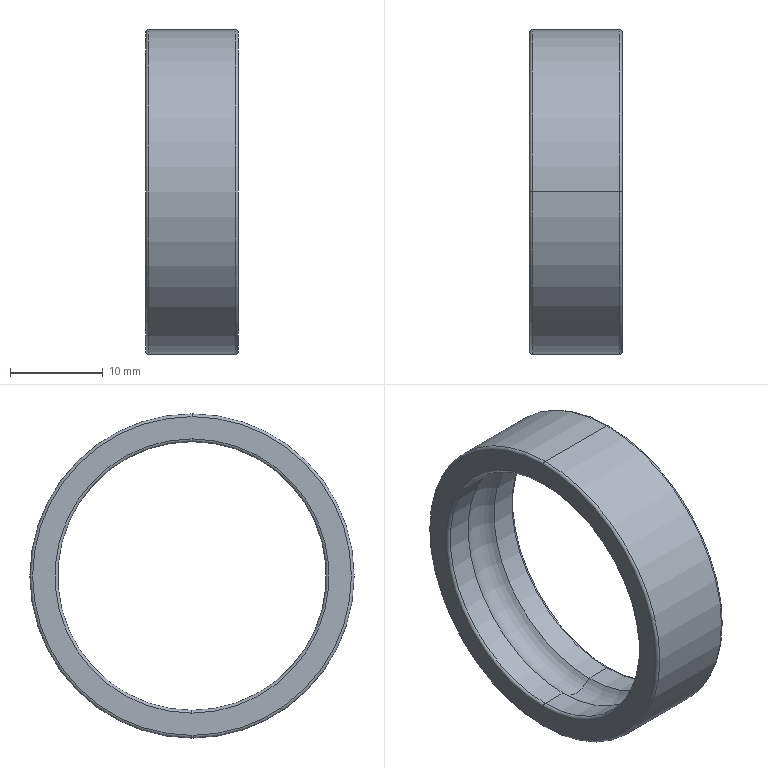Part | SolidWorks | features BaseBody 1 | 1 solid | 18 faces | box 10 x 35 x 35 mm | volume 2757 mm3 | torus 10 | cylinder 6 | plane 2 | commonest cylinder face diameters 29 x4 35 x2
STEP:
#1=CARTESIAN_POINT('',(1.969,0.,14.5));
#2=VERTEX_POINT('',#1);
#3=CARTESIAN_POINT('',(1.969,0.,-14.5));
#4=VERTEX_POINT('',#3);
#5=CARTESIAN_POINT('',(1.969,0.,0.));
#6=DIRECTION('',(1.,0.,0.));
#7=DIRECTION('',(0.,0.,1.));
#8=AXIS2_PLACEMENT_3D('',#5,#6,#7);
#9=CIRCLE('',#8,14.5);
#10=EDGE_CURVE('',#2,#4,#9,.T.);
#11=ORIENTED_EDGE('',*,*,#10,.T.);
#12=CARTESIAN_POINT('',(-1.969,0.,-14.5));
#13=VERTEX_POINT('',#12);
#14=CARTESIAN_POINT('',(0.,0.,-13.));
#15=DIRECTION('',(0.,1.,0.));
#16=DIRECTION('',(0.,0.,1.));
#17=AXIS2_PLACEMENT_3D('',#14,#15,#16);
#18=CIRCLE('',#17,2.475);
#19=EDGE_CURVE('',#4,#13,#18,.T.);
#20=ORIENTED_EDGE('',*,*,#19,.T.);
#21=CARTESIAN_POINT('',(-1.969,0.,14.5));
#22=VERTEX_POINT('',#21);
#23=CARTESIAN_POINT('',(-1.969,0.,0.));
#24=DIRECTION('',(-1.,0.,0.));
#25=DIRECTION('',(0.,0.,-1.));
#26=AXIS2_PLACEMENT_3D('',#23,#24,#25);
#27=CIRCLE('',#26,14.5);
#28=EDGE_CURVE('',#13,#22,#27,.T.);
#29=ORIENTED_EDGE('',*,*,#28,.T.);
#30=CARTESIAN_POINT('',(0.,0.,13.));
#31=DIRECTION('',(0.,-1.,0.));
#32=DIRECTION('',(0.,0.,-1.));
#33=AXIS2_PLACEMENT_3D('',#30,#31,#32);
#34=CIRCLE('',#33,2.475);
#35=EDGE_CURVE('',#2,#22,#34,.T.);
#36=ORIENTED_EDGE('',*,*,#35,.F.);
#37=EDGE_LOOP('',(#11,#20,#29,#36));
#38=FACE_OUTER_BOUND('',#37,.T.);
#39=CARTESIAN_POINT('',(0.,0.,0.));
#40=DIRECTION('',(-1.,0.,0.));
#41=DIRECTION('',(0.,0.,1.));
#42=AXIS2_PLACEMENT_3D('',#39,#40,#41);
#43=TOROIDAL_SURFACE('',#42,13.,2.475);
#44=ADVANCED_FACE('',(#38),#43,.F.);
#45=CARTESIAN_POINT('',(4.7,0.,17.5));
#46=VERTEX_POINT('',#45);
#47=CARTESIAN_POINT('',(4.7,0.,-17.5));
#48=VERTEX_POINT('',#47);
#49=CARTESIAN_POINT('',(4.7,0.,0.));
#50=DIRECTION('',(-1.,0.,0.));
#51=DIRECTION('',(0.,0.,1.));
#52=AXIS2_PLACEMENT_3D('',#49,#50,#51);
#53=CIRCLE('',#52,17.5);
#54=EDGE_CURVE('',#46,#48,#53,.T.);
#55=ORIENTED_EDGE('',*,*,#54,.T.);
#56=CARTESIAN_POINT('',(-4.7,0.,-17.5));
#57=VERTEX_POINT('',#56);
#58=CARTESIAN_POINT('',(-3.5,0.,-17.5));
#59=DIRECTION('',(-1.,0.,0.));
#60=VECTOR('',#59,1000.);
#61=LINE('',#58,#60);
#62=EDGE_CURVE('',#48,#57,#61,.T.);
#63=ORIENTED_EDGE('',*,*,#62,.T.);
#64=CARTESIAN_POINT('',(-4.7,0.,17.5));
#65=VERTEX_POINT('',#64);
#66=CARTESIAN_POINT('',(-4.7,0.,0.));
#67=DIRECTION('',(-1.,0.,0.));
#68=DIRECTION('',(0.,0.,1.));
#69=AXIS2_PLACEMENT_3D('',#66,#67,#68);
#70=CIRCLE('',#69,17.5);
#71=EDGE_CURVE('',#65,#57,#70,.T.);
#72=ORIENTED_EDGE('',*,*,#71,.F.);
#73=CARTESIAN_POINT('',(-3.5,0.,17.5));
#74=DIRECTION('',(-1.,0.,0.));
#75=VECTOR('',#74,1000.);
#76=LINE('',#73,#75);
#77=EDGE_CURVE('',#46,#65,#76,.T.);
#78=ORIENTED_EDGE('',*,*,#77,.F.);
#79=EDGE_LOOP('',(#55,#63,#72,#78));
#80=FACE_OUTER_BOUND('',#79,.T.);
#81=CARTESIAN_POINT('',(-3.5,0.,0.));
#82=DIRECTION('',(-1.,0.,0.));
#83=DIRECTION('',(0.,0.,1.));
#84=AXIS2_PLACEMENT_3D('',#81,#82,#83);
#85=CYLINDRICAL_SURFACE('',#84,17.5);
#86=ADVANCED_FACE('',(#80),#85,.T.);
#87=CARTESIAN_POINT('',(5.,0.,17.2));
#88=VERTEX_POINT('',#87);
#89=CARTESIAN_POINT('',(5.,0.,-17.2));
#90=VERTEX_POINT('',#89);
#91=CARTESIAN_POINT('',(5.,0.,0.));
#92=DIRECTION('',(-1.,0.,0.));
#93=DIRECTION('',(0.,0.,1.));
#94=AXIS2_PLACEMENT_3D('',#91,#92,#93);
#95=CIRCLE('',#94,17.2);
#96=EDGE_CURVE('',#88,#90,#95,.T.);
#97=ORIENTED_EDGE('',*,*,#96,.T.);
#98=CARTESIAN_POINT('',(4.7,0.,-17.2));
#99=DIRECTION('',(0.,1.,0.));
#100=DIRECTION('',(0.,0.,1.));
#101=AXIS2_PLACEMENT_3D('',#98,#99,#100);
#102=CIRCLE('',#101,0.3);
#103=EDGE_CURVE('',#90,#48,#102,.T.);
#104=ORIENTED_EDGE('',*,*,#103,.T.);
#105=ORIENTED_EDGE('',*,*,#54,.F.);
#106=CARTESIAN_POINT('',(4.7,0.,17.2));
#107=DIRECTION('',(0.,-1.,0.));
#108=DIRECTION('',(0.,0.,-1.));
#109=AXIS2_PLACEMENT_3D('',#106,#107,#108);
#110=CIRCLE('',#109,0.3);
#111=EDGE_CURVE('',#88,#46,#110,.T.);
#112=ORIENTED_EDGE('',*,*,#111,.F.);
#113=EDGE_LOOP('',(#97,#104,#105,#112));
#114=FACE_OUTER_BOUND('',#113,.T.);
#115=CARTESIAN_POINT('',(4.7,0.,0.));
#116=DIRECTION('',(-1.,0.,0.));
#117=DIRECTION('',(0.,0.,1.));
#118=AXIS2_PLACEMENT_3D('',#115,#116,#117);
#119=TOROIDAL_SURFACE('',#118,17.2,0.3);
#120=ADVANCED_FACE('',(#114),#119,.T.);
#121=CARTESIAN_POINT('',(4.7,0.,14.5));
#122=VERTEX_POINT('',#121);
#123=CARTESIAN_POINT('',(4.7,0.,-14.5));
#124=VERTEX_POINT('',#123);
#125=CARTESIAN_POINT('',(4.7,0.,0.));
#126=DIRECTION('',(-1.,0.,0.));
#127=DIRECTION('',(0.,0.,1.));
#128=AXIS2_PLACEMENT_3D('',#125,#126,#127);
#129=CIRCLE('',#128,14.5);
#130=EDGE_CURVE('',#122,#124,#129,.T.);
#131=ORIENTED_EDGE('',*,*,#130,.T.);
#132=CARTESIAN_POINT('',(5.,0.,-14.8));
#133=VERTEX_POINT('',#132);
#134=CARTESIAN_POINT('',(4.7,0.,-14.8));
#135=DIRECTION('',(0.,1.,0.));
#136=DIRECTION('',(0.,0.,1.));
#137=AXIS2_PLACEMENT_3D('',#134,#135,#136);
#138=CIRCLE('',#137,0.3);
#139=EDGE_CURVE('',#124,#133,#138,.T.);
#140=ORIENTED_EDGE('',*,*,#139,.T.);
#141=CARTESIAN_POINT('',(5.,0.,14.8));
#142=VERTEX_POINT('',#141);
#143=CARTESIAN_POINT('',(5.,0.,0.));
#144=DIRECTION('',(-1.,0.,0.));
#145=DIRECTION('',(0.,0.,1.));
#146=AXIS2_PLACEMENT_3D('',#143,#144,#145);
#147=CIRCLE('',#146,14.8);
#148=EDGE_CURVE('',#142,#133,#147,.T.);
#149=ORIENTED_EDGE('',*,*,#148,.F.);
#150=CARTESIAN_POINT('',(4.7,0.,14.8));
#151=DIRECTION('',(0.,-1.,0.));
#152=DIRECTION('',(0.,0.,-1.));
#153=AXIS2_PLACEMENT_3D('',#150,#151,#152);
#154=CIRCLE('',#153,0.3);
#155=EDGE_CURVE('',#122,#142,#154,.T.);
#156=ORIENTED_EDGE('',*,*,#155,.F.);
#157=EDGE_LOOP('',(#131,#140,#149,#156));
#158=FACE_OUTER_BOUND('',#157,.T.);
#159=CARTESIAN_POINT('',(4.7,0.,0.));
#160=DIRECTION('',(-1.,0.,0.));
#161=DIRECTION('',(0.,0.,1.));
#162=AXIS2_PLACEMENT_3D('',#159,#160,#161);
#163=TOROIDAL_SURFACE('',#162,14.8,0.3);
#164=ADVANCED_FACE('',(#158),#163,.T.);
#165=CARTESIAN_POINT('',(-5.,0.,14.8));
#166=VERTEX_POINT('',#165);
#167=CARTESIAN_POINT('',(-5.,0.,-14.8));
#168=VERTEX_POINT('',#167);
#169=CARTESIAN_POINT('',(-5.,0.,0.));
#170=DIRECTION('',(-1.,0.,0.));
#171=DIRECTION('',(0.,0.,1.));
#172=AXIS2_PLACEMENT_3D('',#169,#170,#171);
#173=CIRCLE('',#172,14.8);
#174=EDGE_CURVE('',#166,#168,#173,.T.);
#175=ORIENTED_EDGE('',*,*,#174,.T.);
#176=CARTESIAN_POINT('',(-4.7,0.,-14.5));
#177=VERTEX_POINT('',#176);
#178=CARTESIAN_POINT('',(-4.7,0.,-14.8));
#179=DIRECTION('',(0.,1.,0.));
#180=DIRECTION('',(0.,0.,1.));
#181=AXIS2_PLACEMENT_3D('',#178,#179,#180);
#182=CIRCLE('',#181,0.3);
#183=EDGE_CURVE('',#168,#177,#182,.T.);
#184=ORIENTED_EDGE('',*,*,#183,.T.);
#185=CARTESIAN_POINT('',(-4.7,0.,14.5));
#186=VERTEX_POINT('',#185);
#187=CARTESIAN_POINT('',(-4.7,0.,0.));
#188=DIRECTION('',(-1.,0.,0.));
#189=DIRECTION('',(0.,0.,1.));
#190=AXIS2_PLACEMENT_3D('',#187,#188,#189);
#191=CIRCLE('',#190,14.5);
#192=EDGE_CURVE('',#186,#177,#191,.T.);
#193=ORIENTED_EDGE('',*,*,#192,.F.);
#194=CARTESIAN_POINT('',(-4.7,0.,14.8));
#195=DIRECTION('',(0.,-1.,0.));
#196=DIRECTION('',(0.,0.,-1.));
#197=AXIS2_PLACEMENT_3D('',#194,#195,#196);
#198=CIRCLE('',#197,0.3);
#199=EDGE_CURVE('',#166,#186,#198,.T.);
#200=ORIENTED_EDGE('',*,*,#199,.F.);
#201=EDGE_LOOP('',(#175,#184,#193,#200));
#202=FACE_OUTER_BOUND('',#201,.T.);
#203=CARTESIAN_POINT('',(-4.7,0.,0.));
#204=DIRECTION('',(-1.,0.,0.));
#205=DIRECTION('',(0.,0.,1.));
#206=AXIS2_PLACEMENT_3D('',#203,#204,#205);
#207=TOROIDAL_SURFACE('',#206,14.8,0.3);
#208=ADVANCED_FACE('',(#202),#207,.T.);
#209=ORIENTED_EDGE('',*,*,#71,.T.);
#210=CARTESIAN_POINT('',(-5.,0.,-17.2));
#211=VERTEX_POINT('',#210);
#212=CARTESIAN_POINT('',(-4.7,0.,-17.2));
#213=DIRECTION('',(0.,1.,0.));
#214=DIRECTION('',(0.,0.,1.));
#215=AXIS2_PLACEMENT_3D('',#212,#213,#214);
#216=CIRCLE('',#215,0.3);
#217=EDGE_CURVE('',#57,#211,#216,.T.);
#218=ORIENTED_EDGE('',*,*,#217,.T.);
#219=CARTESIAN_POINT('',(-5.,0.,17.2));
#220=VERTEX_POINT('',#219);
#221=CARTESIAN_POINT('',(-5.,0.,0.));
#222=DIRECTION('',(-1.,0.,0.));
#223=DIRECTION('',(0.,0.,1.));
#224=AXIS2_PLACEMENT_3D('',#221,#222,#223);
#225=CIRCLE('',#224,17.2);
#226=EDGE_CURVE('',#220,#211,#225,.T.);
#227=ORIENTED_EDGE('',*,*,#226,.F.);
#228=CARTESIAN_POINT('',(-4.7,0.,17.2));
#229=DIRECTION('',(0.,-1.,0.));
#230=DIRECTION('',(0.,0.,-1.));
#231=AXIS2_PLACEMENT_3D('',#228,#229,#230);
#232=CIRCLE('',#231,0.3);
#233=EDGE_CURVE('',#65,#220,#232,.T.);
#234=ORIENTED_EDGE('',*,*,#233,.F.);
#235=EDGE_LOOP('',(#209,#218,#227,#234));
#236=FACE_OUTER_BOUND('',#235,.T.);
#237=CARTESIAN_POINT('',(-4.7,0.,0.));
#238=DIRECTION('',(-1.,0.,0.));
#239=DIRECTION('',(0.,0.,1.));
#240=AXIS2_PLACEMENT_3D('',#237,#238,#239);
#241=TOROIDAL_SURFACE('',#240,17.2,0.3);
#242=ADVANCED_FACE('',(#236),#241,.T.);
#243=CARTESIAN_POINT('',(4.7,0.,0.));
#244=DIRECTION('',(-1.,0.,0.));
#245=DIRECTION('',(0.,0.,1.));
#246=AXIS2_PLACEMENT_3D('',#243,#244,#245);
#247=CIRCLE('',#246,14.5);
#248=EDGE_CURVE('',#124,#122,#247,.T.);
#249=ORIENTED_EDGE('',*,*,#248,.F.);
#250=CARTESIAN_POINT('',(-3.5,0.,-14.5));
#251=DIRECTION('',(-1.,0.,0.));
#252=VECTOR('',#251,1000.);
#253=LINE('',#250,#252);
#254=EDGE_CURVE('',#124,#4,#253,.T.);
#255=ORIENTED_EDGE('',*,*,#254,.T.);
#256=ORIENTED_EDGE('',*,*,#10,.F.);
#257=CARTESIAN_POINT('',(-3.5,0.,14.5));
#258=DIRECTION('',(-1.,0.,0.));
#259=VECTOR('',#258,1000.);
#260=LINE('',#257,#259);
#261=EDGE_CURVE('',#122,#2,#260,.T.);
#262=ORIENTED_EDGE('',*,*,#261,.F.);
#263=EDGE_LOOP('',(#249,#255,#256,#262));
#264=FACE_OUTER_BOUND('',#263,.T.);
#265=CARTESIAN_POINT('',(-3.5,0.,0.));
#266=DIRECTION('',(-1.,0.,0.));
#267=DIRECTION('',(0.,0.,1.));
#268=AXIS2_PLACEMENT_3D('',#265,#266,#267);
#269=CYLINDRICAL_SURFACE('',#268,14.5);
#270=ADVANCED_FACE('',(#264),#269,.F.);
#271=ORIENTED_EDGE('',*,*,#28,.F.);
#272=CARTESIAN_POINT('',(-3.5,0.,-14.5));
#273=DIRECTION('',(-1.,0.,0.));
#274=VECTOR('',#273,1000.);
#275=LINE('',#272,#274);
#276=EDGE_CURVE('',#13,#177,#275,.T.);
#277=ORIENTED_EDGE('',*,*,#276,.T.);
#278=CARTESIAN_POINT('',(-4.7,0.,0.));
#279=DIRECTION('',(-1.,0.,0.));
#280=DIRECTION('',(0.,0.,1.));
#281=AXIS2_PLACEMENT_3D('',#278,#279,#280);
#282=CIRCLE('',#281,14.5);
#283=EDGE_CURVE('',#177,#186,#282,.T.);
#284=ORIENTED_EDGE('',*,*,#283,.T.);
#285=CARTESIAN_POINT('',(-3.5,0.,14.5));
#286=DIRECTION('',(-1.,0.,0.));
#287=VECTOR('',#286,1000.);
#288=LINE('',#285,#287);
#289=EDGE_CURVE('',#22,#186,#288,.T.);
#290=ORIENTED_EDGE('',*,*,#289,.F.);
#291=EDGE_LOOP('',(#271,#277,#284,#290));
#292=FACE_OUTER_BOUND('',#291,.T.);
#293=CARTESIAN_POINT('',(-3.5,0.,0.));
#294=DIRECTION('',(-1.,0.,0.));
#295=DIRECTION('',(0.,0.,1.));
#296=AXIS2_PLACEMENT_3D('',#293,#294,#295);
#297=CYLINDRICAL_SURFACE('',#296,14.5);
#298=ADVANCED_FACE('',(#292),#297,.F.);
#299=ORIENTED_EDGE('',*,*,#148,.T.);
#300=CARTESIAN_POINT('',(5.,0.,0.));
#301=DIRECTION('',(-1.,0.,0.));
#302=DIRECTION('',(0.,0.,1.));
#303=AXIS2_PLACEMENT_3D('',#300,#301,#302);
#304=CIRCLE('',#303,14.8);
#305=EDGE_CURVE('',#133,#142,#304,.T.);
#306=ORIENTED_EDGE('',*,*,#305,.T.);
#307=EDGE_LOOP('',(#299,#306));
#308=FACE_BOUND('',#307,.T.);
#309=ORIENTED_EDGE('',*,*,#96,.F.);
#310=CARTESIAN_POINT('',(5.,0.,0.));
#311=DIRECTION('',(-1.,0.,0.));
#312=DIRECTION('',(0.,0.,1.));
#313=AXIS2_PLACEMENT_3D('',#310,#311,#312);
#314=CIRCLE('',#313,17.2);
#315=EDGE_CURVE('',#90,#88,#314,.T.);
#316=ORIENTED_EDGE('',*,*,#315,.F.);
#317=EDGE_LOOP('',(#309,#316));
#318=FACE_OUTER_BOUND('',#317,.T.);
#319=CARTESIAN_POINT('',(5.,17.2,0.));
#320=DIRECTION('',(-1.,0.,0.));
#321=DIRECTION('',(0.,0.,1.));
#322=AXIS2_PLACEMENT_3D('',#319,#320,#321);
#323=PLANE('',#322);
#324=ADVANCED_FACE('',(#308,#318),#323,.F.);
#325=ORIENTED_EDGE('',*,*,#174,.F.);
#326=CARTESIAN_POINT('',(-5.,0.,0.));
#327=DIRECTION('',(-1.,0.,0.));
#328=DIRECTION('',(0.,0.,1.));
#329=AXIS2_PLACEMENT_3D('',#326,#327,#328);
#330=CIRCLE('',#329,14.8);
#331=EDGE_CURVE('',#168,#166,#330,.T.);
#332=ORIENTED_EDGE('',*,*,#331,.F.);
#333=EDGE_LOOP('',(#325,#332));
#334=FACE_BOUND('',#333,.T.);
#335=ORIENTED_EDGE('',*,*,#226,.T.);
#336=CARTESIAN_POINT('',(-5.,0.,0.));
#337=DIRECTION('',(-1.,0.,0.));
#338=DIRECTION('',(0.,0.,1.));
#339=AXIS2_PLACEMENT_3D('',#336,#337,#338);
#340=CIRCLE('',#339,17.2);
#341=EDGE_CURVE('',#211,#220,#340,.T.);
#342=ORIENTED_EDGE('',*,*,#341,.T.);
#343=EDGE_LOOP('',(#335,#342));
#344=FACE_OUTER_BOUND('',#343,.T.);
#345=CARTESIAN_POINT('',(-5.,17.2,0.));
#346=DIRECTION('',(1.,0.,0.));
#347=DIRECTION('',(0.,1.,0.));
#348=AXIS2_PLACEMENT_3D('',#345,#346,#347);
#349=PLANE('',#348);
#350=ADVANCED_FACE('',(#334,#344),#349,.F.);
#351=ORIENTED_EDGE('',*,*,#276,.F.);
#352=CARTESIAN_POINT('',(-1.969,0.,0.));
#353=DIRECTION('',(-1.,0.,0.));
#354=DIRECTION('',(0.,0.,-1.));
#355=AXIS2_PLACEMENT_3D('',#352,#353,#354);
#356=CIRCLE('',#355,14.5);
#357=EDGE_CURVE('',#22,#13,#356,.T.);
#358=ORIENTED_EDGE('',*,*,#357,.F.);
#359=ORIENTED_EDGE('',*,*,#289,.T.);
#360=ORIENTED_EDGE('',*,*,#192,.T.);
#361=EDGE_LOOP('',(#351,#358,#359,#360));
#362=FACE_OUTER_BOUND('',#361,.T.);
#363=CARTESIAN_POINT('',(-3.5,0.,0.));
#364=DIRECTION('',(-1.,0.,0.));
#365=DIRECTION('',(0.,0.,1.));
#366=AXIS2_PLACEMENT_3D('',#363,#364,#365);
#367=CYLINDRICAL_SURFACE('',#366,14.5);
#368=ADVANCED_FACE('',(#362),#367,.F.);
#369=ORIENTED_EDGE('',*,*,#254,.F.);
#370=ORIENTED_EDGE('',*,*,#130,.F.);
#371=ORIENTED_EDGE('',*,*,#261,.T.);
#372=CARTESIAN_POINT('',(1.969,0.,0.));
#373=DIRECTION('',(1.,0.,0.));
#374=DIRECTION('',(0.,0.,1.));
#375=AXIS2_PLACEMENT_3D('',#372,#373,#374);
#376=CIRCLE('',#375,14.5);
#377=EDGE_CURVE('',#4,#2,#376,.T.);
#378=ORIENTED_EDGE('',*,*,#377,.F.);
#379=EDGE_LOOP('',(#369,#370,#371,#378));
#380=FACE_OUTER_BOUND('',#379,.T.);
#381=CARTESIAN_POINT('',(-3.5,0.,0.));
#382=DIRECTION('',(-1.,0.,0.));
#383=DIRECTION('',(0.,0.,1.));
#384=AXIS2_PLACEMENT_3D('',#381,#382,#383);
#385=CYLINDRICAL_SURFACE('',#384,14.5);
#386=ADVANCED_FACE('',(#380),#385,.F.);
#387=ORIENTED_EDGE('',*,*,#217,.F.);
#388=CARTESIAN_POINT('',(-4.7,0.,0.));
#389=DIRECTION('',(-1.,0.,0.));
#390=DIRECTION('',(0.,0.,1.));
#391=AXIS2_PLACEMENT_3D('',#388,#389,#390);
#392=CIRCLE('',#391,17.5);
#393=EDGE_CURVE('',#57,#65,#392,.T.);
#394=ORIENTED_EDGE('',*,*,#393,.T.);
#395=ORIENTED_EDGE('',*,*,#233,.T.);
#396=ORIENTED_EDGE('',*,*,#341,.F.);
#397=EDGE_LOOP('',(#387,#394,#395,#396));
#398=FACE_OUTER_BOUND('',#397,.T.);
#399=CARTESIAN_POINT('',(-4.7,0.,0.));
#400=DIRECTION('',(-1.,0.,0.));
#401=DIRECTION('',(0.,0.,1.));
#402=AXIS2_PLACEMENT_3D('',#399,#400,#401);
#403=TOROIDAL_SURFACE('',#402,17.2,0.3);
#404=ADVANCED_FACE('',(#398),#403,.T.);
#405=ORIENTED_EDGE('',*,*,#183,.F.);
#406=ORIENTED_EDGE('',*,*,#331,.T.);
#407=ORIENTED_EDGE('',*,*,#199,.T.);
#408=ORIENTED_EDGE('',*,*,#283,.F.);
#409=EDGE_LOOP('',(#405,#406,#407,#408));
#410=FACE_OUTER_BOUND('',#409,.T.);
#411=CARTESIAN_POINT('',(-4.7,0.,0.));
#412=DIRECTION('',(-1.,0.,0.));
#413=DIRECTION('',(0.,0.,1.));
#414=AXIS2_PLACEMENT_3D('',#411,#412,#413);
#415=TOROIDAL_SURFACE('',#414,14.8,0.3);
#416=ADVANCED_FACE('',(#410),#415,.T.);
#417=ORIENTED_EDGE('',*,*,#139,.F.);
#418=ORIENTED_EDGE('',*,*,#248,.T.);
#419=ORIENTED_EDGE('',*,*,#155,.T.);
#420=ORIENTED_EDGE('',*,*,#305,.F.);
#421=EDGE_LOOP('',(#417,#418,#419,#420));
#422=FACE_OUTER_BOUND('',#421,.T.);
#423=CARTESIAN_POINT('',(4.7,0.,0.));
#424=DIRECTION('',(-1.,0.,0.));
#425=DIRECTION('',(0.,0.,1.));
#426=AXIS2_PLACEMENT_3D('',#423,#424,#425);
#427=TOROIDAL_SURFACE('',#426,14.8,0.3);
#428=ADVANCED_FACE('',(#422),#427,.T.);
#429=ORIENTED_EDGE('',*,*,#103,.F.);
#430=ORIENTED_EDGE('',*,*,#315,.T.);
#431=ORIENTED_EDGE('',*,*,#111,.T.);
#432=CARTESIAN_POINT('',(4.7,0.,0.));
#433=DIRECTION('',(-1.,0.,0.));
#434=DIRECTION('',(0.,0.,1.));
#435=AXIS2_PLACEMENT_3D('',#432,#433,#434);
#436=CIRCLE('',#435,17.5);
#437=EDGE_CURVE('',#48,#46,#436,.T.);
#438=ORIENTED_EDGE('',*,*,#437,.F.);
#439=EDGE_LOOP('',(#429,#430,#431,#438));
#440=FACE_OUTER_BOUND('',#439,.T.);
#441=CARTESIAN_POINT('',(4.7,0.,0.));
#442=DIRECTION('',(-1.,0.,0.));
#443=DIRECTION('',(0.,0.,1.));
#444=AXIS2_PLACEMENT_3D('',#441,#442,#443);
#445=TOROIDAL_SURFACE('',#444,17.2,0.3);
#446=ADVANCED_FACE('',(#440),#445,.T.);
#447=ORIENTED_EDGE('',*,*,#62,.F.);
#448=ORIENTED_EDGE('',*,*,#437,.T.);
#449=ORIENTED_EDGE('',*,*,#77,.T.);
#450=ORIENTED_EDGE('',*,*,#393,.F.);
#451=EDGE_LOOP('',(#447,#448,#449,#450));
#452=FACE_OUTER_BOUND('',#451,.T.);
#453=CARTESIAN_POINT('',(-3.5,0.,0.));
#454=DIRECTION('',(-1.,0.,0.));
#455=DIRECTION('',(0.,0.,1.));
#456=AXIS2_PLACEMENT_3D('',#453,#454,#455);
#457=CYLINDRICAL_SURFACE('',#456,17.5);
#458=ADVANCED_FACE('',(#452),#457,.T.);
#459=ORIENTED_EDGE('',*,*,#19,.F.);
#460=ORIENTED_EDGE('',*,*,#377,.T.);
#461=ORIENTED_EDGE('',*,*,#35,.T.);
#462=ORIENTED_EDGE('',*,*,#357,.T.);
#463=EDGE_LOOP('',(#459,#460,#461,#462));
#464=FACE_OUTER_BOUND('',#463,.T.);
#465=CARTESIAN_POINT('',(0.,0.,0.));
#466=DIRECTION('',(-1.,0.,0.));
#467=DIRECTION('',(0.,0.,1.));
#468=AXIS2_PLACEMENT_3D('',#465,#466,#467);
#469=TOROIDAL_SURFACE('',#468,13.,2.475);
#470=ADVANCED_FACE('',(#464),#469,.F.);
#471=CLOSED_SHELL('',(#44,#86,#120,#164,#208,#242,#270,#298,#324,#350,#368,#386,#404,#416,#428,#446,#458,#470));
#472=MANIFOLD_SOLID_BREP('',#471);
#473=CARTESIAN_POINT('',(0.,0.,0.));
#474=DIRECTION('',(0.,0.,1.));
#475=DIRECTION('',(1.,0.,0.));
#476=AXIS2_PLACEMENT_3D('',#473,#474,#475);
#477=(LENGTH_UNIT()NAMED_UNIT(*)SI_UNIT(.MILLI.,.METRE.));
#478=UNCERTAINTY_MEASURE_WITH_UNIT(LENGTH_MEASURE(0.00001),#477,'','');
#479=(NAMED_UNIT(*)PLANE_ANGLE_UNIT()SI_UNIT($,.RADIAN.));
#480=(NAMED_UNIT(*)SI_UNIT($,.STERADIAN.)SOLID_ANGLE_UNIT());
#481=(GEOMETRIC_REPRESENTATION_CONTEXT(3)GLOBAL_UNCERTAINTY_ASSIGNED_CONTEXT((#478))GLOBAL_UNIT_ASSIGNED_CONTEXT((#477,#479,#480))REPRESENTATION_CONTEXT('',''));
#482=ADVANCED_BREP_SHAPE_REPRESENTATION('',(#472,#476),#481);